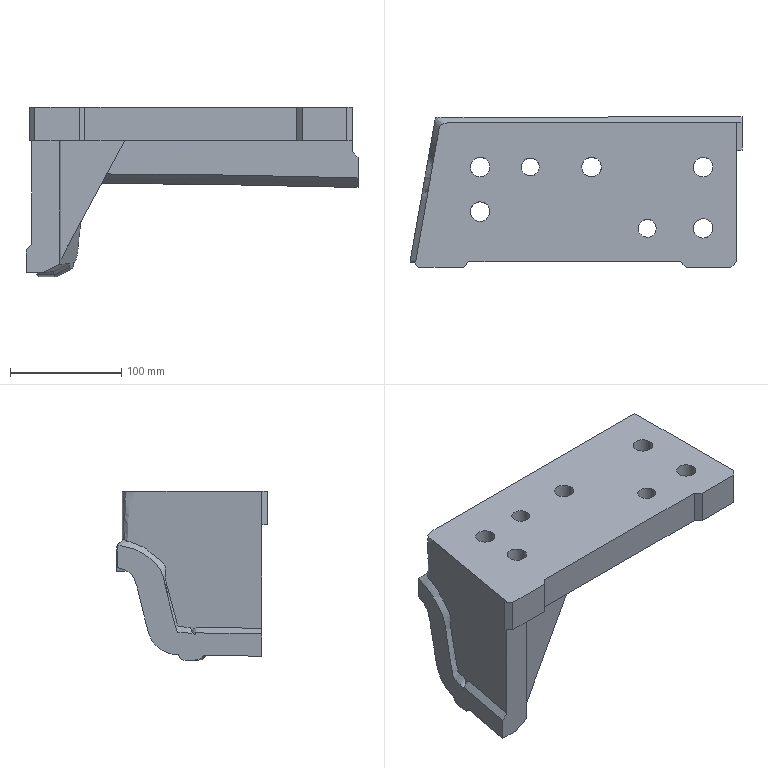Part | NX | features solid 2 | 1 solid | 45 faces | box 297.945 x 135.312 x 152.223 mm | volume 1640303 mm3 | plane 23 | cylinder 12 | spline 10 | commonest cylinder face diameters 17.5 x5 25 x5 16 x2